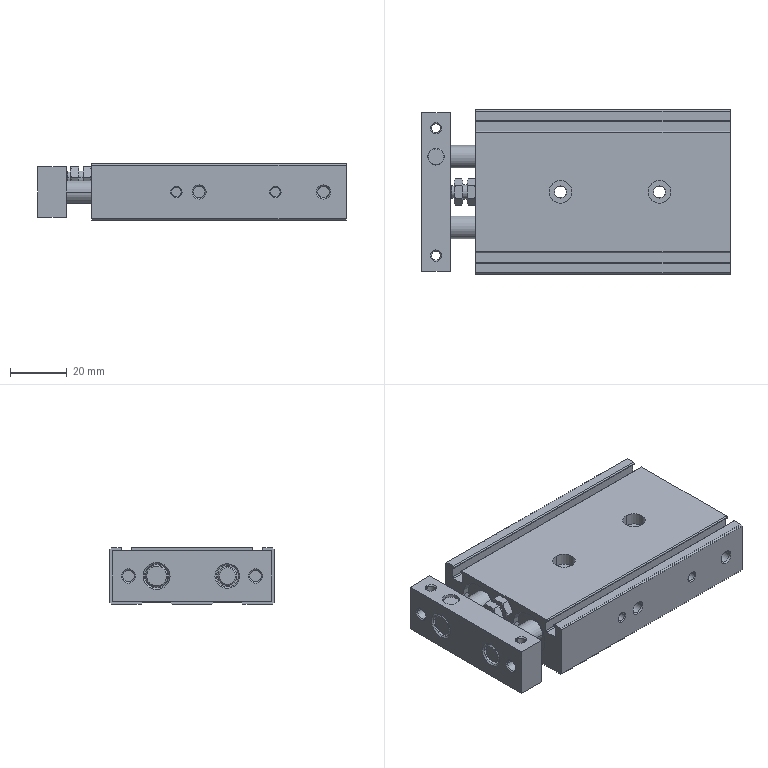Part | SolidWorks | 2 solids | 260 faces | box 109 x 58 x 20 mm | volume 97636 mm3 | cylinder 98 | plane 83 | cone 79 | commonest cylinder face diameters 3.242 x16 4.134 x16 8 x14 0.8 x12 16 x12 0.4 x4